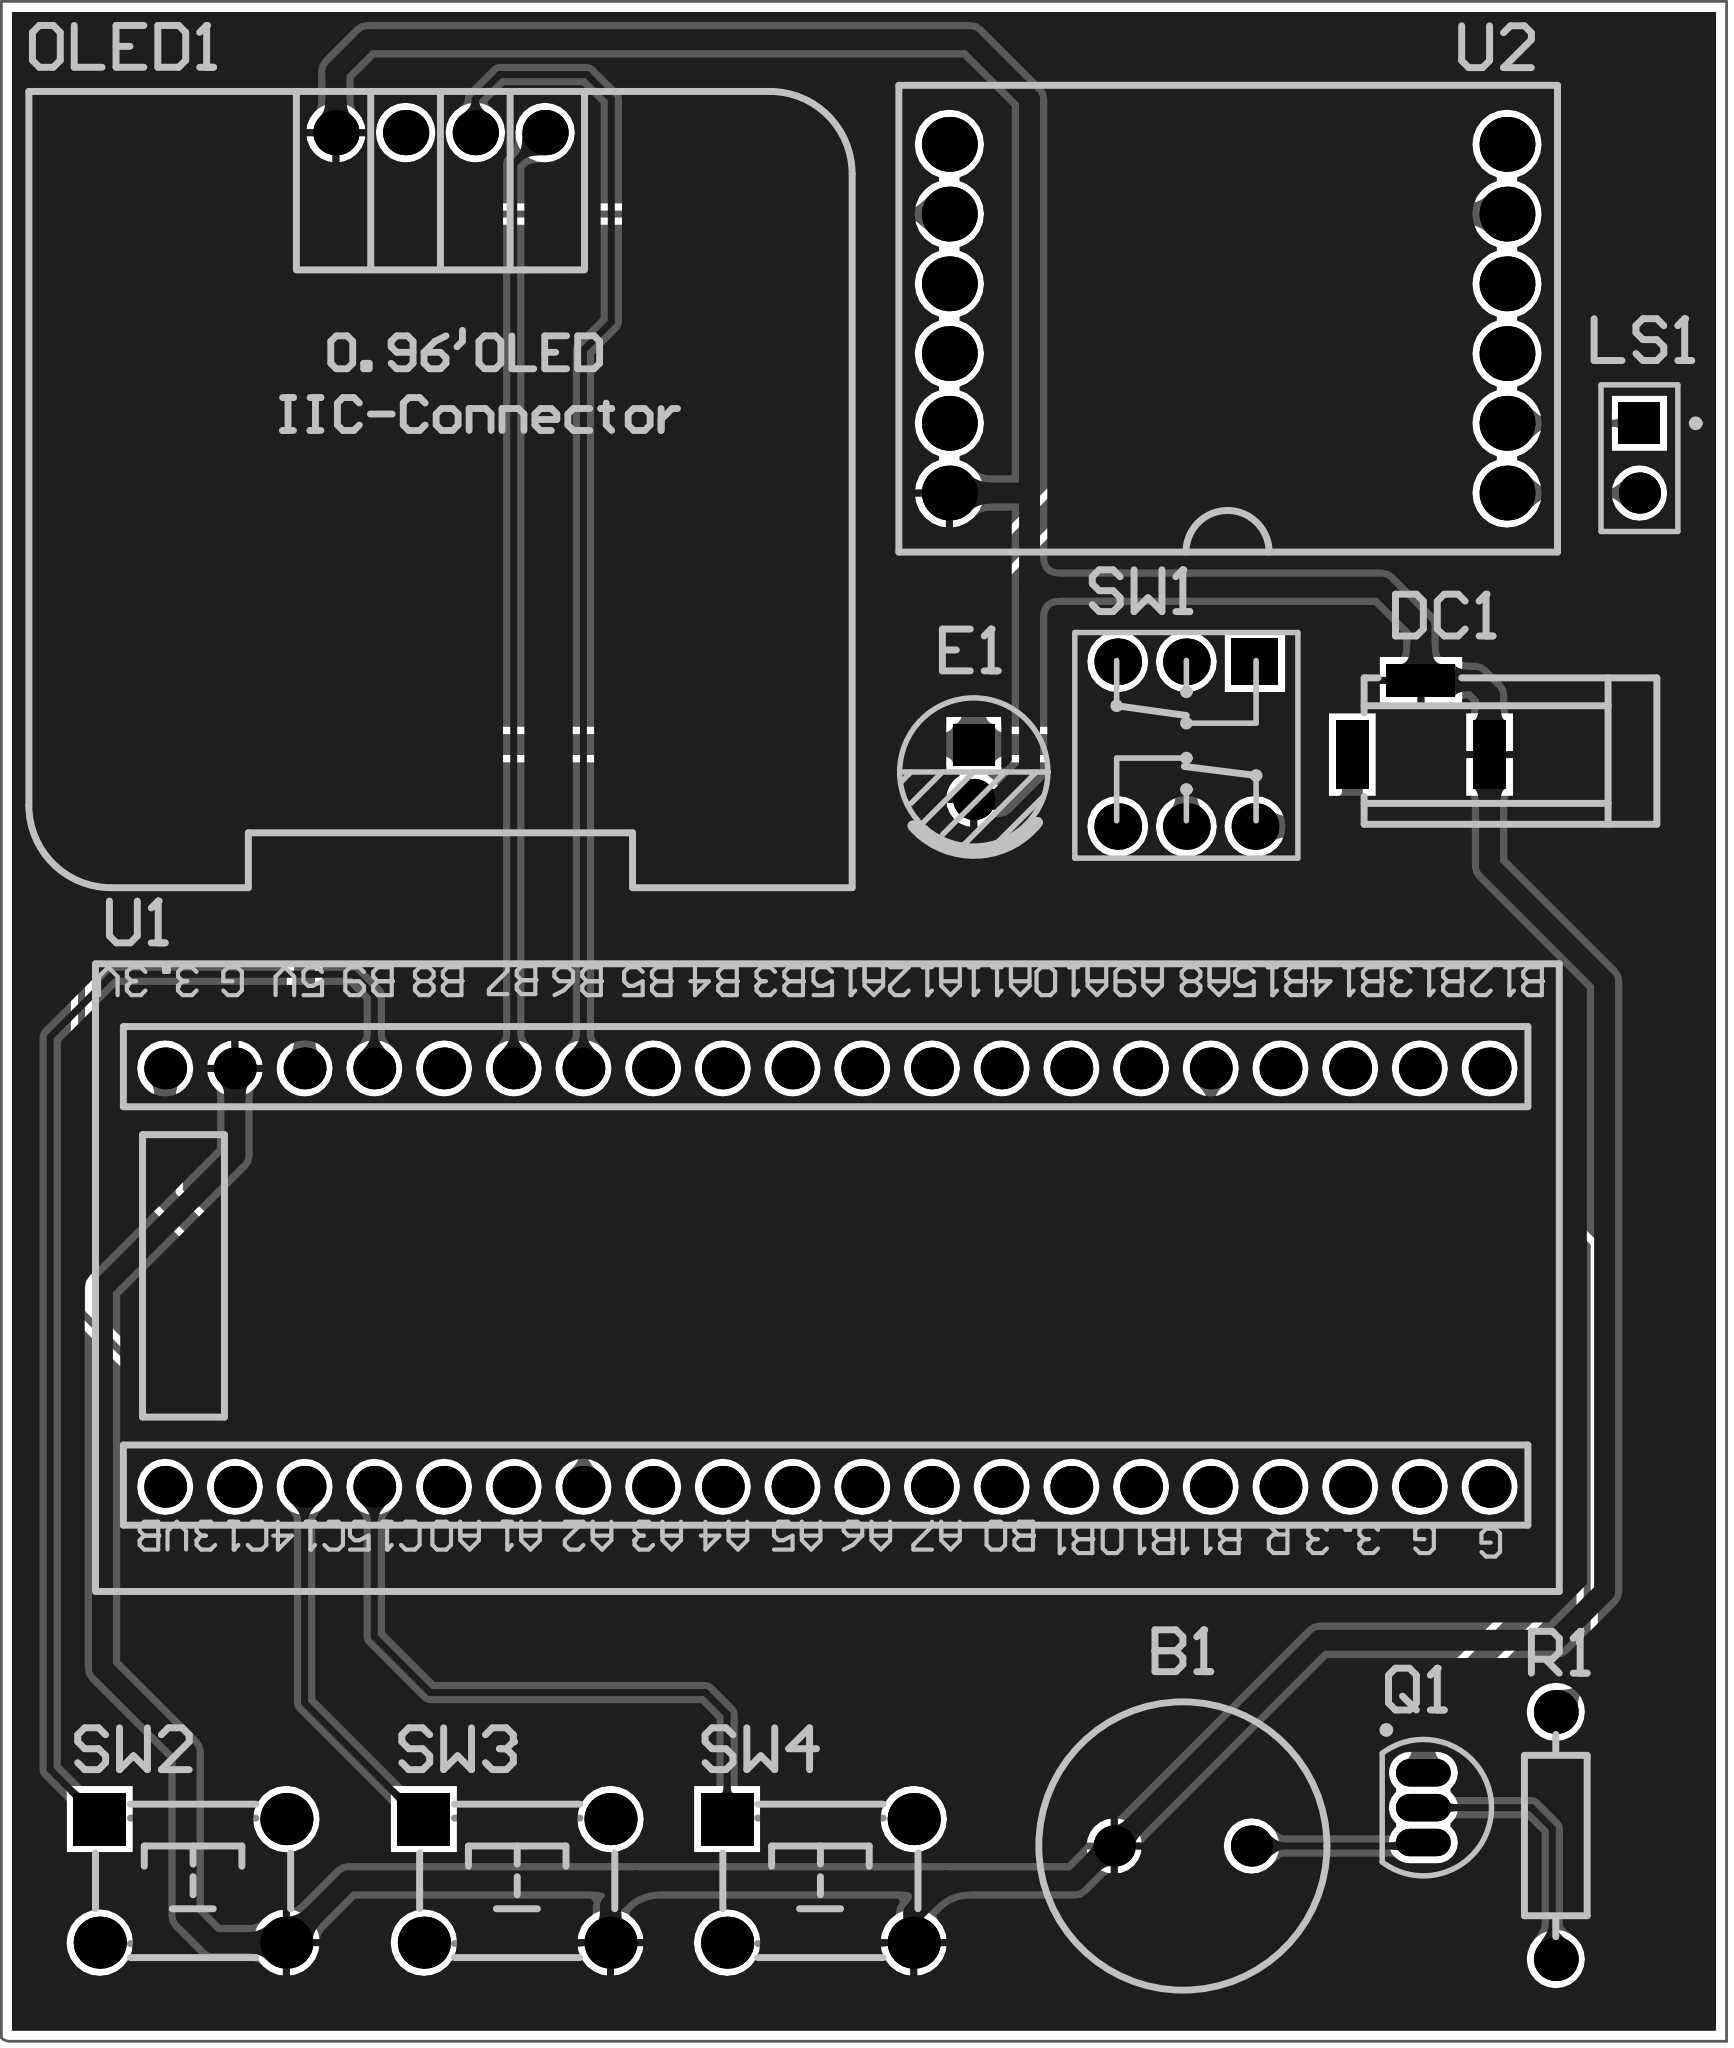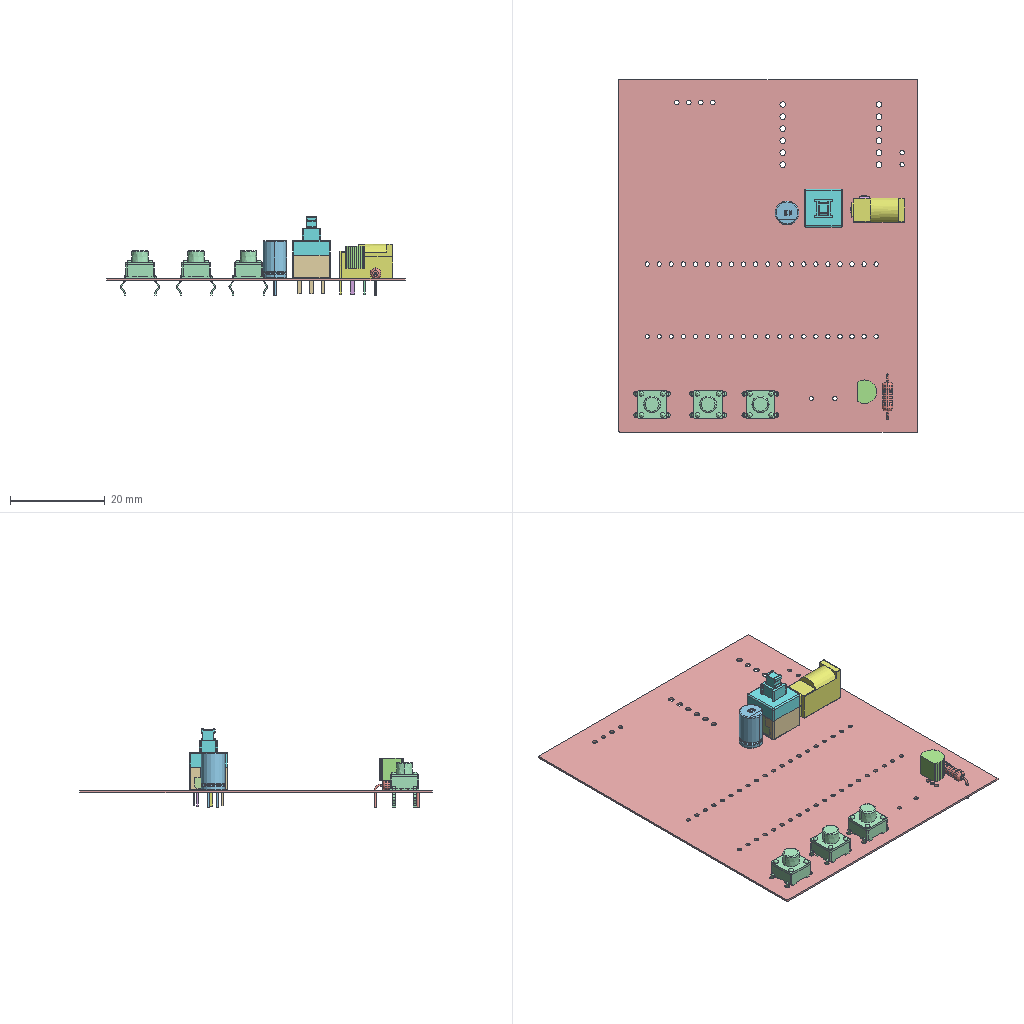Circuit board layout | Altium Designer | box 62.9 x 74.3 x 16.6 mm
Layer stack:
# Altium Designer layer stack of  (unit mm; dielectric type: 0 none, 1 core, 2 prepreg, 3 surface material)
index,name,kind,layer,copper_thickness_mm,dielectric_type,dielectric_thickness_mm,dielectric_material,dielectric_constant
0,Top Paste,other,,,,,,
1,Top Overlay,other,,,,,,
2,Top Solder,dielectric,,,3,0.0102,Solder Resist,3.5
3,Top Layer,copper,Top Layer,0.0356,,,,
4,Dielectric 1,dielectric,,,0,0.32,FR-4,4.8
5,Bottom Layer,copper,Bottom Layer,0.0356,,,,
6,Bottom Solder,dielectric,,,3,0.0102,Solder Resist,3.5
7,Bottom Overlay,other,,,,,,
8,Bottom Paste,other,,,,,,
# drill layer pairs: low layer,high layer
drill_pair,Top Layer,Bottom Layer
Part placement:
Designator,Comment,Layer,Footprint,Center-X(mm),Center-Y(mm),Rotation
U2,MY1680U-12P_1,TopLayer,COMM-TH_MY1680-12P,124.079,91.948,360
U1,STM32F103C8T6 minimum system board,TopLayer,STM32核心板,109.474,57.023,90
SW1,KET 8X8,TopLayer,KFT_DIP-8X8,122.555,76.454,180
SW2,6x6x5,TopLayer,TSW_DIP-6*6*6,86.36,35.052,0
SW3,6x6x5,TopLayer,TSW_DIP-6*6*6,98.171,35.052,0
SW4,6x6x5,TopLayer,TSW_DIP-6*6*6,109.22,35.052,0
R1,1K,TopLayer,RS_1/4W,136.017,36.703,270
Q1,9012,TopLayer,TO-92A,131.191,37.719,180
OLED1,0.96OLED_4P_MODULE_JX,TopLayer,0.96OLED_4P,95.376,98.724,0
LS1,Speaker,TopLayer,PIN2,139.065,86.868,270
E1,470uF,TopLayer,CS_2.0*5*8_-_C,114.808,75.438,90
DC1,DC_Socket,TopLayer,DC-002,131.104,77.423,360
B1,Motor,TopLayer,RB5-10.5,122.428,36.322,180
Pad and via stacks:
# Altium Designer via and pad stacks of  (unit mm). Each distinct definition once, with the count of objects using it.
# via: kind,start_layer,end_layer,hole_mm,diameter_mm,mode(0 simple;1 top-mid-bottom;2 full stack),diameter_per_layer,count,example_net
# pad: kind,layer,hole_mm,hole_type(0 round;1 square;2 slot),plating,top_size,top_shape(1 round;2 rect;3 octagon;9 rounded rect),mid_size,bottom_size,mode,footprint,size_per_layer,count,example
pad,Multi-Layer,0.9,0,plated,1.7x1.7,1,1.7x1.7,1.7x1.7,0,KFT DIP-8X8,,5,SW1.6
pad,Multi-Layer,0.9,0,plated,1.7x1.7,2,1.7x1.7,1.7x1.7,0,KFT DIP-8X8,,1,SW1.1
pad,Multi-Layer,0.6,2,plated,2.5x1.2,2,2.5x1.2,2.5x1.2,0,DC-002,,3,DC1.3
pad,Multi-Layer,0.9144,2,plated,1.524x1.524,1,1.524x1.524,1.524x1.524,0,STM32\u00BA\u00CB\u00D0\u00C4\u00B0\u00E5,,40,U1.1
pad,Multi-Layer,1,2,plated,1.65x1.65,1,1.65x1.65,1.65x1.65,0,0.96OLED_4P,,4,OLED1.1
pad,Multi-Layer,0.6,0,plated,1.6x1.6,1,1.6x1.6,1.6x1.6,0,RS 1/4W,,2,R1.2
pad,Multi-Layer,0.9,0,plated,2x1,1,2x1,2x1,0,TO-92A,,3,Q1.3
pad,Multi-Layer,0.9,0,plated,1.5x1.5,1,1.5x1.5,1.5x1.5,0,RB5-10.5,,2,B1.1
pad,Multi-Layer,1,0,plated,1.9x1.9,1,1.9x1.9,1.9x1.9,0,TSW DIP-6*6*6,,9,SW2.4
pad,Multi-Layer,1,0,plated,1.9x1.9,2,1.9x1.9,1.9x1.9,0,TSW DIP-6*6*6,,3,SW2.1
pad,Multi-Layer,1.2,0,plated,2x2,1,2x2,2x2,0,COMM-TH_MY1680-12P,,12,U2.1
pad,Multi-Layer,0.9,0,plated,1.5x1.5,2,1.5x1.5,1.5x1.5,0,PIN2,,1,LS1.1
pad,Multi-Layer,0.9,0,plated,1.5x1.5,1,1.5x1.5,1.5x1.5,0,PIN2,,1,LS1.2
pad,Multi-Layer,0.8,0,plated,1.5x1.5,2,1.5x1.5,1.5x1.5,0,CS 2.0*5*8 - C,,1,E1.1
pad,Multi-Layer,0.8,0,plated,1.5x1.5,1,1.5x1.5,1.5x1.5,0,CS 2.0*5*8 - C,,1,E1.2
Copper pours:
name,layer,net,type(0 solid;1 hatched;2 none)
D,Bottom Layer,GND,0
D,Top Layer,GND,0
Design rules, without the lines most boards share:
# Altium Designer design rules of  (exported by Altium Designer, unit mm)
# columns: name | kind | enabled | priority | scope1 | scope2 | descriptor | typed fields (field=value)
ShortCircuit | 15 | enabled | 1 | All | All | Short-Circuit Constraint (Allowed=Yes) (All),(All) |
Clearance | 0 | enabled | 1 | All | All | Clearance Constraint (Gap=10mil) (All),(All) | gap=0.254
PlaneConnect | 6 | enabled | 1 | All | All | Power Plane Connect Rule(Relief Connect )(Expansion=20mil) (Conductor Width=10mil) (Air Gap=10mil) (Entries=4) (All) | relief_conductor_width=0.254 relief_entries=4 relief_expansion=0.508
PolygonConnect | 20 | enabled | 1 | All | All | Polygon Connect Rule(Relief Connect )(Conductor Width=10mil) (Relief Angle=90 Angle) (Entries=4) (Air Gap Width=10mil) (All),(All) | connect_style(0=relief,1=direct,2=none)=0 relief_conductor_width=0.254 relief_entries=4
Width | 2 | enabled | 1 | All | All | Width Constraint (Min=10mil) (Max=30mil) (Preferred=10mil) (All) |
RoutingVias | 11 | enabled | 1 | All | All | Routing Via (MinHoleWidth=28mil) (MaxHoleWidth=28mil) (PreferredHoleWidth=28mil) (MinWidth=50mil) (MaxWidth=50mil) (PreferedWidth=50mil) (All) | via_min_hole=0.7112 via_max_hole=0.7112 via_preferred_diameter=1.27 via_preferred_hole=0.7112
PasteMaskExpansion | 14 | enabled | 1 | All | All | Paste Mask Expansion (Expansion =0mil) (All) | expansion=0
SolderMaskExpansion | 13 | enabled | 1 | All | All | Solder Mask Expansion (Expansion =4mil) (All) | expansion=0.1016
DiffPairsRouting | 51 | enabled | 1 | All | All | Differential Pairs Uncoupled Length using the Gap Constraints (Min=10mil) (Max=10mil) (Prefered=10mil)  and Width Constraints (Min=15mil) (Max=15mil) (Prefered=15mil) (All) |
HoleToHoleClearance | 52 | enabled | 1 | All | All | Hole To Hole Clearance (Gap=10mil) (All),(All) | gap=0.254
MinimumSolderMaskSliver | 53 | enabled | 1 | All | All | Minimum Solder Mask Sliver (Gap=0mil) (All),(All) |
SilkToSolderMaskClearance | 54 | enabled | 1 | IsPad | All | Silk To Solder Mask (Clearance=0mil) (IsPad),(All) |
SilkToSilkClearance | 55 | enabled | 1 | All | All | Silk to Silk (Clearance=0mil) (All),(All) |
Classes set for this board:
# Altium Designer classes of  (member kind: 0 net, 1 component, 2 from-to, 3 pad, 4 layer, 5 differential pair, 6 design channel, 7 polygon, 8 structure, 9 xSignal)
# columns: class name | member kind | superclass | members
Sheet1 | 1 | no | OLED1; U1; SW1; SW2; SW3; DC1; SW4; B1; SW3; Q1; SW2; U2; E1; R1; LS1; SW1;